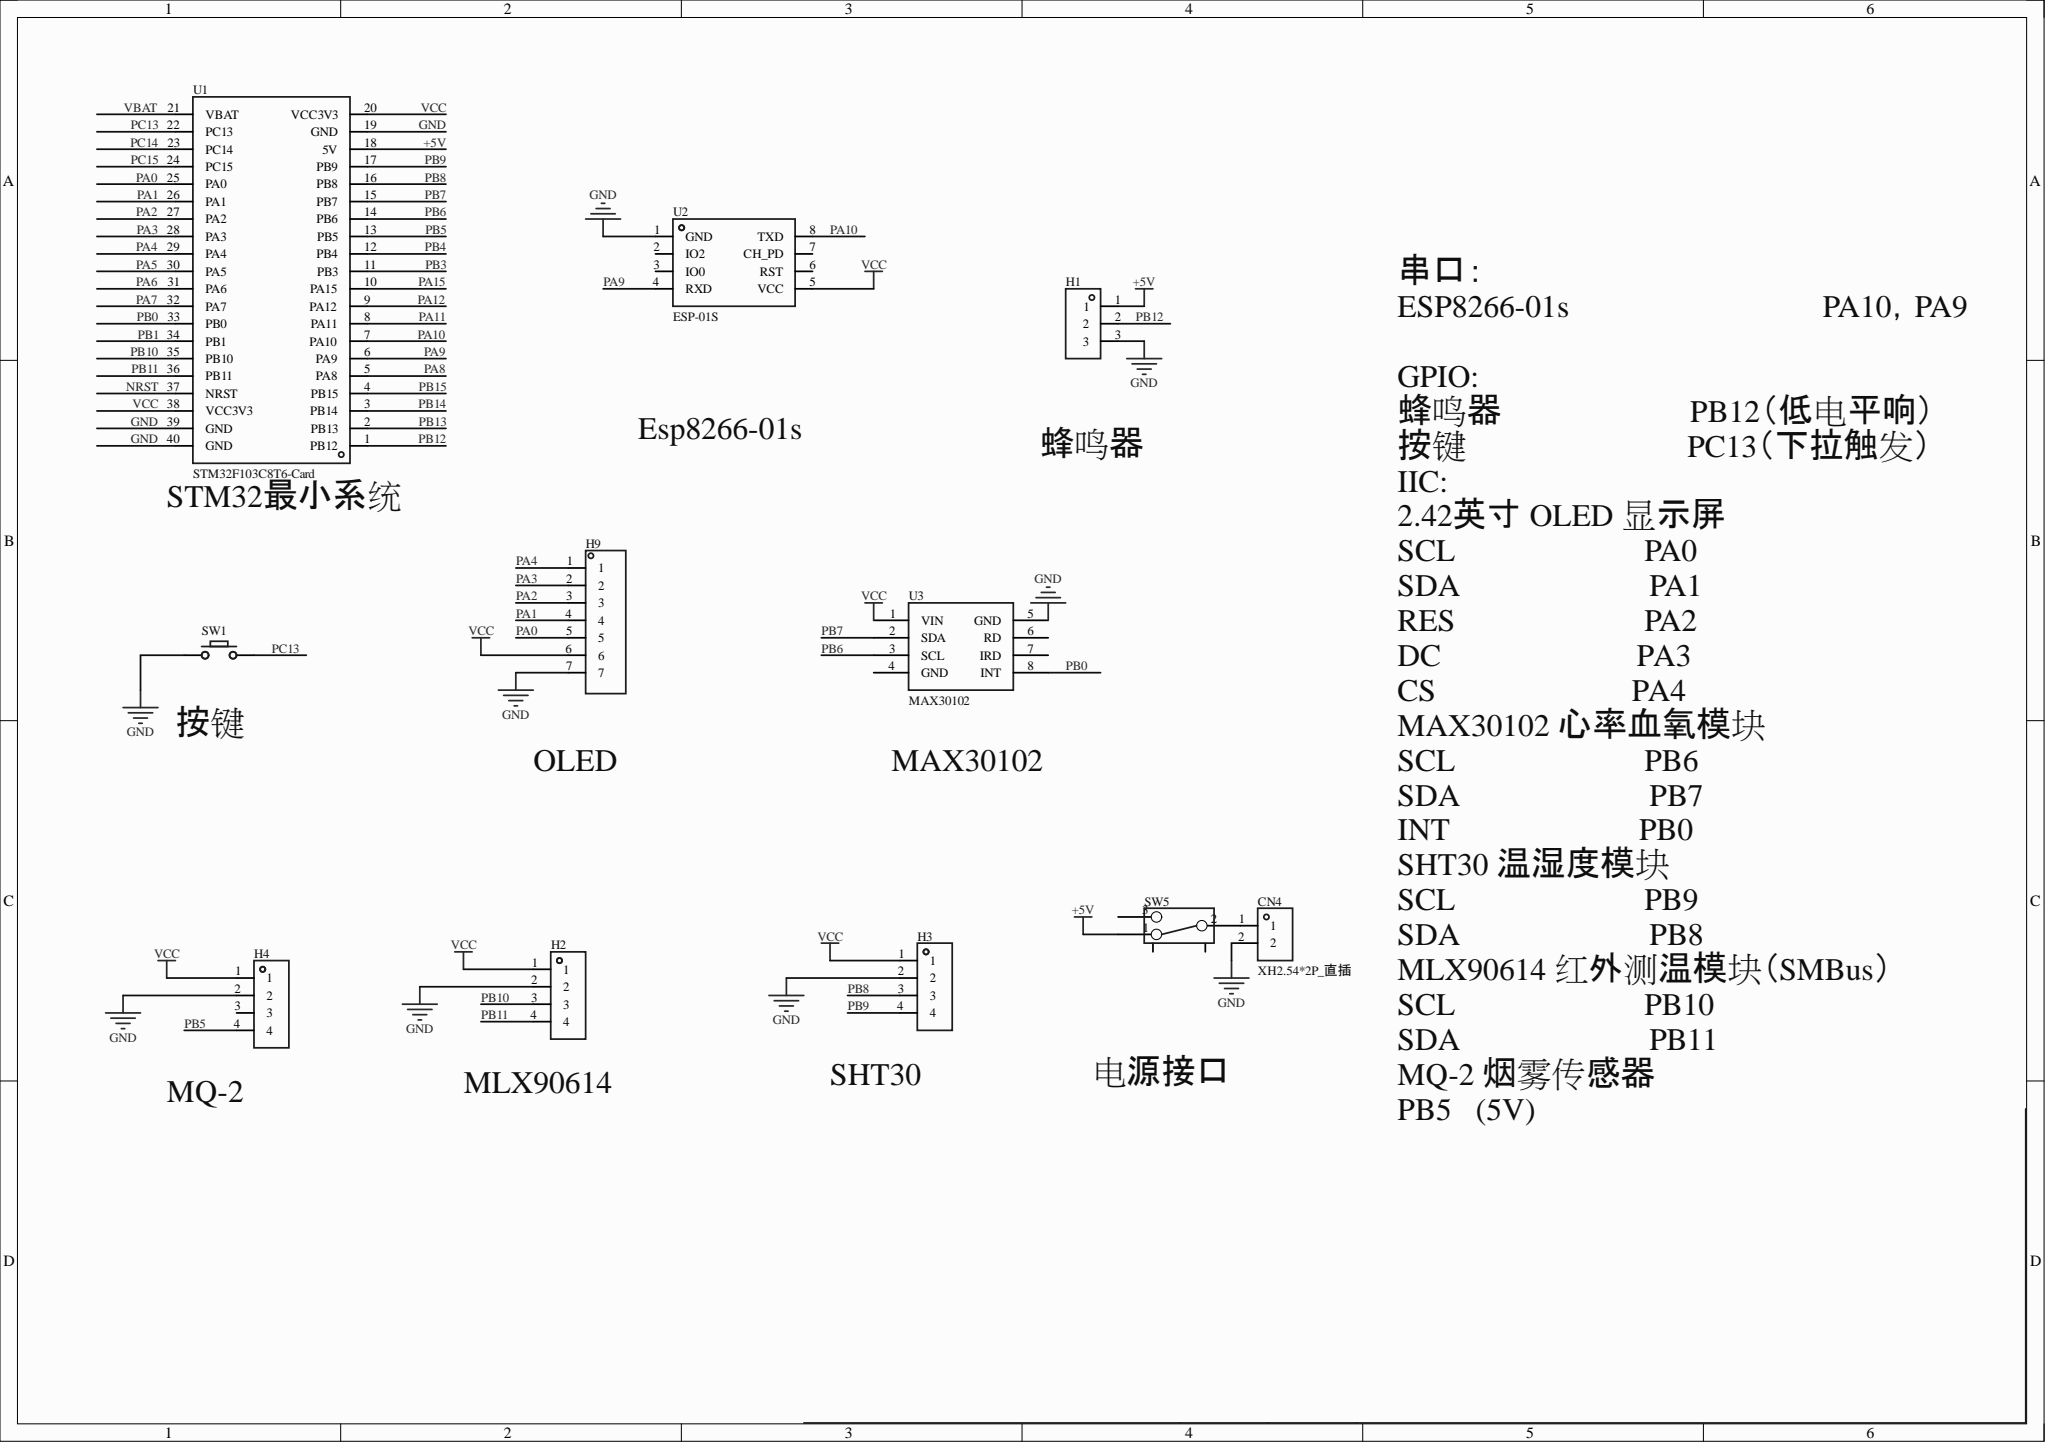Circuit board | Altium Designer | 11 parts | 21 nets
Bill of materials:
Comment,Description,Designator,Footprint,LibRef,Quantity
"XH2.54*2P_直插","","CN4","CONN-TH_2P-P2.50-XH2.54-2P","XH2.54*2P_直插","1"
"","","H1","HDR-TH_3P-P2.54-V-F","HDR-F_2.54_1x3P","1"
"","","H2, H3, H4","HDR-TH_4P-P2.54-V-F","HDR-F_2.54_1x4P","3"
"","","H9","HDR-TH_7P-P2.54-V-F","HDR-F_2.54_1x7P","1"
"","","SW1","Key_TH_3.5x6x4.3","Key_TH_3.5x6x4.3","1"
"","","SW5","拨动开关","拨动开关_正","1"
"STM32F103C8T6-Card","","U1","CONN-TH_L53.3-W22.9_STM32F103C8T6-CARD","STM32F103C8T6-Card","1"
"ESP-01S","","U2","WIFIM-TH_ESP-01S","ESP-01S_C111009","1"
"MAX30102","","U3","MAX30102","MAX30102","1"
Netlist (Protel format):
[
CN4
CONN-TH_2P-P2.50-XH2.54-2P
XH2.54*2P_直插



]
[
H1
HDR-TH_3P-P2.54-V-F




]
[
H2
HDR-TH_4P-P2.54-V-F




]
[
H3
HDR-TH_4P-P2.54-V-F




]
[
H4
HDR-TH_4P-P2.54-V-F




]
[
H9
HDR-TH_7P-P2.54-V-F




]
[
SW1
Key_TH_3.5x6x4.3




]
[
SW5
拨动开关




]
[
U1
CONN-TH_L53.3-W22.9_STM32F103C8T6-CARD
STM32F103C8T6-Card



]
[
U2
WIFIM-TH_ESP-01S
ESP-01S



]
[
U3
MAX30102
MAX30102



]
(
VCC
H2-1
H3-1
H4-1
H9-6
U1-20
U1-38
U2-5
U3-1
)
(
PC13
SW1-B
U1-22
)
(
PB12
H1-2
U1-1
)
(
PB11
H2-4
U1-36
)
(
PB10
H2-3
U1-35
)
(
PB9
H3-4
U1-17
)
(
PB8
H3-3
U1-16
)
(
PB7
U1-15
U3-2
)
(
PB6
U1-14
U3-3
)
(
PB5
H4-4
U1-13
)
(
PB0
U1-33
U3-8
)
(
PA10
U1-7
U2-8
)
(
PA9
U1-6
U2-4
)
(
PA4
H9-1
U1-29
)
(
PA3
H9-2
U1-28
)
(
PA2
H9-3
U1-27
)
(
PA1
H9-4
U1-26
)
(
PA0
H9-5
U1-25
)
(
NetCN4_1
CN4-1
SW5-2
)
(
GND
CN4-2
H1-3
H2-2
H3-2
H4-2
H9-7
SW1-A
U1-19
U1-39
U1-40
U2-1
U3-5
)
(
+5V
H1-1
SW5-1
U1-18
)